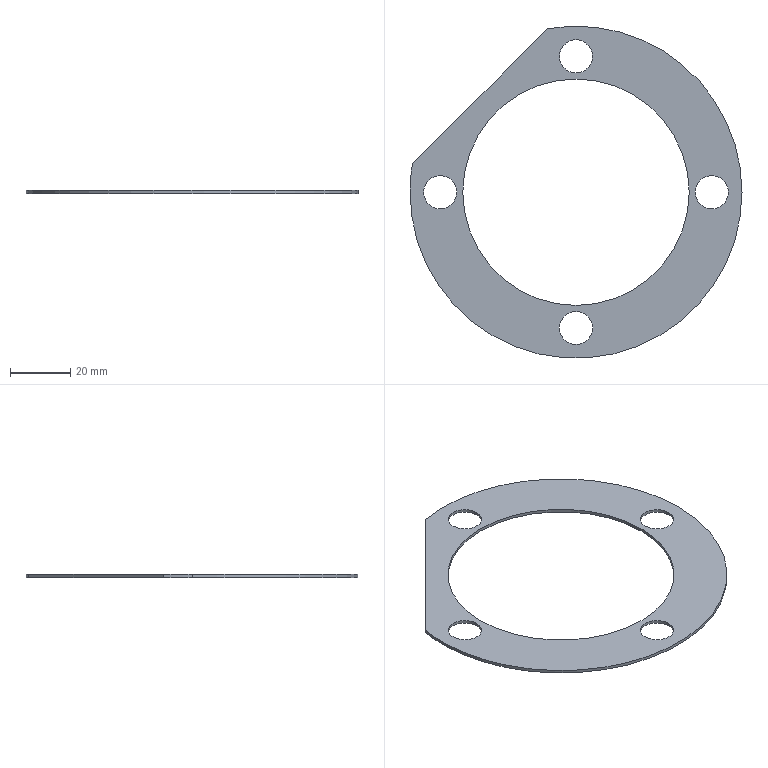Part | SolidWorks | features BaseBody 1 | 1 solid | 16 faces | box 110 x 110 x 1 mm | volume 4275 mm3 | cylinder 13 | plane 3 | commonest cylinder face diameters 11 x8 110 x3 75 x2
STEP:
#1=CARTESIAN_POINT('',(15.5,0.,0.));
#2=VERTEX_POINT('',#1);
#3=CARTESIAN_POINT('',(4.5,0.,0.));
#4=VERTEX_POINT('',#3);
#5=CARTESIAN_POINT('',(10.,0.,0.));
#6=DIRECTION('',(0.,0.,-1.));
#7=DIRECTION('',(1.,0.,0.));
#8=AXIS2_PLACEMENT_3D('',#5,#6,#7);
#9=CIRCLE('',#8,5.5);
#10=EDGE_CURVE('',#2,#4,#9,.T.);
#11=ORIENTED_EDGE('',*,*,#10,.T.);
#12=CARTESIAN_POINT('',(4.5,0.,1.));
#13=VERTEX_POINT('',#12);
#14=CARTESIAN_POINT('',(4.5,0.,0.));
#15=DIRECTION('',(0.,0.,1.));
#16=VECTOR('',#15,1000.);
#17=LINE('',#14,#16);
#18=EDGE_CURVE('',#4,#13,#17,.T.);
#19=ORIENTED_EDGE('',*,*,#18,.T.);
#20=CARTESIAN_POINT('',(15.5,0.,1.));
#21=VERTEX_POINT('',#20);
#22=CARTESIAN_POINT('',(10.,0.,1.));
#23=DIRECTION('',(0.,0.,-1.));
#24=DIRECTION('',(1.,0.,0.));
#25=AXIS2_PLACEMENT_3D('',#22,#23,#24);
#26=CIRCLE('',#25,5.5);
#27=EDGE_CURVE('',#21,#13,#26,.T.);
#28=ORIENTED_EDGE('',*,*,#27,.F.);
#29=CARTESIAN_POINT('',(15.5,0.,0.));
#30=DIRECTION('',(0.,0.,1.));
#31=VECTOR('',#30,1000.);
#32=LINE('',#29,#31);
#33=EDGE_CURVE('',#2,#21,#32,.T.);
#34=ORIENTED_EDGE('',*,*,#33,.F.);
#35=EDGE_LOOP('',(#11,#19,#28,#34));
#36=FACE_OUTER_BOUND('',#35,.T.);
#37=CARTESIAN_POINT('',(10.,0.,0.));
#38=DIRECTION('',(0.,0.,1.));
#39=DIRECTION('',(1.,0.,0.));
#40=AXIS2_PLACEMENT_3D('',#37,#38,#39);
#41=CYLINDRICAL_SURFACE('',#40,5.5);
#42=ADVANCED_FACE('',(#36),#41,.F.);
#43=CARTESIAN_POINT('',(60.5,45.,0.));
#44=VERTEX_POINT('',#43);
#45=CARTESIAN_POINT('',(49.5,45.,0.));
#46=VERTEX_POINT('',#45);
#47=CARTESIAN_POINT('',(55.,45.,0.));
#48=DIRECTION('',(0.,0.,-1.));
#49=DIRECTION('',(1.,0.,0.));
#50=AXIS2_PLACEMENT_3D('',#47,#48,#49);
#51=CIRCLE('',#50,5.5);
#52=EDGE_CURVE('',#44,#46,#51,.T.);
#53=ORIENTED_EDGE('',*,*,#52,.T.);
#54=CARTESIAN_POINT('',(49.5,45.,1.));
#55=VERTEX_POINT('',#54);
#56=CARTESIAN_POINT('',(49.5,45.,0.));
#57=DIRECTION('',(0.,0.,1.));
#58=VECTOR('',#57,1000.);
#59=LINE('',#56,#58);
#60=EDGE_CURVE('',#46,#55,#59,.T.);
#61=ORIENTED_EDGE('',*,*,#60,.T.);
#62=CARTESIAN_POINT('',(60.5,45.,1.));
#63=VERTEX_POINT('',#62);
#64=CARTESIAN_POINT('',(55.,45.,1.));
#65=DIRECTION('',(0.,0.,-1.));
#66=DIRECTION('',(1.,0.,0.));
#67=AXIS2_PLACEMENT_3D('',#64,#65,#66);
#68=CIRCLE('',#67,5.5);
#69=EDGE_CURVE('',#63,#55,#68,.T.);
#70=ORIENTED_EDGE('',*,*,#69,.F.);
#71=CARTESIAN_POINT('',(60.5,45.,0.));
#72=DIRECTION('',(0.,0.,1.));
#73=VECTOR('',#72,1000.);
#74=LINE('',#71,#73);
#75=EDGE_CURVE('',#44,#63,#74,.T.);
#76=ORIENTED_EDGE('',*,*,#75,.F.);
#77=EDGE_LOOP('',(#53,#61,#70,#76));
#78=FACE_OUTER_BOUND('',#77,.T.);
#79=CARTESIAN_POINT('',(55.,45.,0.));
#80=DIRECTION('',(0.,0.,1.));
#81=DIRECTION('',(1.,0.,0.));
#82=AXIS2_PLACEMENT_3D('',#79,#80,#81);
#83=CYLINDRICAL_SURFACE('',#82,5.5);
#84=ADVANCED_FACE('',(#78),#83,.F.);
#85=CARTESIAN_POINT('',(105.5,0.,0.));
#86=VERTEX_POINT('',#85);
#87=CARTESIAN_POINT('',(94.5,0.,0.));
#88=VERTEX_POINT('',#87);
#89=CARTESIAN_POINT('',(100.,0.,0.));
#90=DIRECTION('',(0.,0.,-1.));
#91=DIRECTION('',(1.,0.,0.));
#92=AXIS2_PLACEMENT_3D('',#89,#90,#91);
#93=CIRCLE('',#92,5.5);
#94=EDGE_CURVE('',#86,#88,#93,.T.);
#95=ORIENTED_EDGE('',*,*,#94,.T.);
#96=CARTESIAN_POINT('',(94.5,0.,1.));
#97=VERTEX_POINT('',#96);
#98=CARTESIAN_POINT('',(94.5,0.,0.));
#99=DIRECTION('',(0.,0.,1.));
#100=VECTOR('',#99,1000.);
#101=LINE('',#98,#100);
#102=EDGE_CURVE('',#88,#97,#101,.T.);
#103=ORIENTED_EDGE('',*,*,#102,.T.);
#104=CARTESIAN_POINT('',(105.5,0.,1.));
#105=VERTEX_POINT('',#104);
#106=CARTESIAN_POINT('',(100.,0.,1.));
#107=DIRECTION('',(0.,0.,-1.));
#108=DIRECTION('',(1.,0.,0.));
#109=AXIS2_PLACEMENT_3D('',#106,#107,#108);
#110=CIRCLE('',#109,5.5);
#111=EDGE_CURVE('',#105,#97,#110,.T.);
#112=ORIENTED_EDGE('',*,*,#111,.F.);
#113=CARTESIAN_POINT('',(105.5,0.,0.));
#114=DIRECTION('',(0.,0.,1.));
#115=VECTOR('',#114,1000.);
#116=LINE('',#113,#115);
#117=EDGE_CURVE('',#86,#105,#116,.T.);
#118=ORIENTED_EDGE('',*,*,#117,.F.);
#119=EDGE_LOOP('',(#95,#103,#112,#118));
#120=FACE_OUTER_BOUND('',#119,.T.);
#121=CARTESIAN_POINT('',(100.,0.,0.));
#122=DIRECTION('',(0.,0.,1.));
#123=DIRECTION('',(1.,0.,0.));
#124=AXIS2_PLACEMENT_3D('',#121,#122,#123);
#125=CYLINDRICAL_SURFACE('',#124,5.5);
#126=ADVANCED_FACE('',(#120),#125,.F.);
#127=CARTESIAN_POINT('',(60.5,-45.,0.));
#128=VERTEX_POINT('',#127);
#129=CARTESIAN_POINT('',(49.5,-45.,0.));
#130=VERTEX_POINT('',#129);
#131=CARTESIAN_POINT('',(55.,-45.,0.));
#132=DIRECTION('',(0.,0.,-1.));
#133=DIRECTION('',(1.,0.,0.));
#134=AXIS2_PLACEMENT_3D('',#131,#132,#133);
#135=CIRCLE('',#134,5.5);
#136=EDGE_CURVE('',#128,#130,#135,.T.);
#137=ORIENTED_EDGE('',*,*,#136,.T.);
#138=CARTESIAN_POINT('',(49.5,-45.,1.));
#139=VERTEX_POINT('',#138);
#140=CARTESIAN_POINT('',(49.5,-45.,0.));
#141=DIRECTION('',(0.,0.,1.));
#142=VECTOR('',#141,1000.);
#143=LINE('',#140,#142);
#144=EDGE_CURVE('',#130,#139,#143,.T.);
#145=ORIENTED_EDGE('',*,*,#144,.T.);
#146=CARTESIAN_POINT('',(60.5,-45.,1.));
#147=VERTEX_POINT('',#146);
#148=CARTESIAN_POINT('',(55.,-45.,1.));
#149=DIRECTION('',(0.,0.,-1.));
#150=DIRECTION('',(1.,0.,0.));
#151=AXIS2_PLACEMENT_3D('',#148,#149,#150);
#152=CIRCLE('',#151,5.5);
#153=EDGE_CURVE('',#147,#139,#152,.T.);
#154=ORIENTED_EDGE('',*,*,#153,.F.);
#155=CARTESIAN_POINT('',(60.5,-45.,0.));
#156=DIRECTION('',(0.,0.,1.));
#157=VECTOR('',#156,1000.);
#158=LINE('',#155,#157);
#159=EDGE_CURVE('',#128,#147,#158,.T.);
#160=ORIENTED_EDGE('',*,*,#159,.F.);
#161=EDGE_LOOP('',(#137,#145,#154,#160));
#162=FACE_OUTER_BOUND('',#161,.T.);
#163=CARTESIAN_POINT('',(55.,-45.,0.));
#164=DIRECTION('',(0.,0.,1.));
#165=DIRECTION('',(1.,0.,0.));
#166=AXIS2_PLACEMENT_3D('',#163,#164,#165);
#167=CYLINDRICAL_SURFACE('',#166,5.5);
#168=ADVANCED_FACE('',(#162),#167,.F.);
#169=CARTESIAN_POINT('',(92.5,0.,0.));
#170=VERTEX_POINT('',#169);
#171=CARTESIAN_POINT('',(17.5,0.,0.));
#172=VERTEX_POINT('',#171);
#173=CARTESIAN_POINT('',(55.,0.,0.));
#174=DIRECTION('',(0.,0.,-1.));
#175=DIRECTION('',(1.,0.,0.));
#176=AXIS2_PLACEMENT_3D('',#173,#174,#175);
#177=CIRCLE('',#176,37.5);
#178=EDGE_CURVE('',#170,#172,#177,.T.);
#179=ORIENTED_EDGE('',*,*,#178,.T.);
#180=CARTESIAN_POINT('',(17.5,0.,1.));
#181=VERTEX_POINT('',#180);
#182=CARTESIAN_POINT('',(17.5,0.,0.));
#183=DIRECTION('',(0.,0.,1.));
#184=VECTOR('',#183,1000.);
#185=LINE('',#182,#184);
#186=EDGE_CURVE('',#172,#181,#185,.T.);
#187=ORIENTED_EDGE('',*,*,#186,.T.);
#188=CARTESIAN_POINT('',(92.5,0.,1.));
#189=VERTEX_POINT('',#188);
#190=CARTESIAN_POINT('',(55.,0.,1.));
#191=DIRECTION('',(0.,0.,-1.));
#192=DIRECTION('',(1.,0.,0.));
#193=AXIS2_PLACEMENT_3D('',#190,#191,#192);
#194=CIRCLE('',#193,37.5);
#195=EDGE_CURVE('',#189,#181,#194,.T.);
#196=ORIENTED_EDGE('',*,*,#195,.F.);
#197=CARTESIAN_POINT('',(92.5,0.,0.));
#198=DIRECTION('',(0.,0.,1.));
#199=VECTOR('',#198,1000.);
#200=LINE('',#197,#199);
#201=EDGE_CURVE('',#170,#189,#200,.T.);
#202=ORIENTED_EDGE('',*,*,#201,.F.);
#203=EDGE_LOOP('',(#179,#187,#196,#202));
#204=FACE_OUTER_BOUND('',#203,.T.);
#205=CARTESIAN_POINT('',(55.,0.,0.));
#206=DIRECTION('',(0.,0.,1.));
#207=DIRECTION('',(1.,0.,0.));
#208=AXIS2_PLACEMENT_3D('',#205,#206,#207);
#209=CYLINDRICAL_SURFACE('',#208,37.5);
#210=ADVANCED_FACE('',(#204),#209,.F.);
#211=CARTESIAN_POINT('',(0.8195,9.459,0.));
#212=VERTEX_POINT('',#211);
#213=CARTESIAN_POINT('',(0.,0.,0.));
#214=VERTEX_POINT('',#213);
#215=CARTESIAN_POINT('',(55.,0.,0.));
#216=DIRECTION('',(0.,0.,1.));
#217=DIRECTION('',(1.,0.,0.));
#218=AXIS2_PLACEMENT_3D('',#215,#216,#217);
#219=CIRCLE('',#218,55.);
#220=EDGE_CURVE('',#212,#214,#219,.T.);
#221=ORIENTED_EDGE('',*,*,#220,.T.);
#222=CARTESIAN_POINT('',(0.,0.,1.));
#223=VERTEX_POINT('',#222);
#224=CARTESIAN_POINT('',(0.,0.,0.));
#225=DIRECTION('',(0.,0.,1.));
#226=VECTOR('',#225,1000.);
#227=LINE('',#224,#226);
#228=EDGE_CURVE('',#214,#223,#227,.T.);
#229=ORIENTED_EDGE('',*,*,#228,.T.);
#230=CARTESIAN_POINT('',(0.8195,9.459,1.));
#231=VERTEX_POINT('',#230);
#232=CARTESIAN_POINT('',(55.,0.,1.));
#233=DIRECTION('',(0.,0.,-1.));
#234=DIRECTION('',(1.,0.,0.));
#235=AXIS2_PLACEMENT_3D('',#232,#233,#234);
#236=CIRCLE('',#235,55.);
#237=EDGE_CURVE('',#223,#231,#236,.T.);
#238=ORIENTED_EDGE('',*,*,#237,.T.);
#239=CARTESIAN_POINT('',(0.8195,9.459,0.));
#240=DIRECTION('',(0.,0.,1.));
#241=VECTOR('',#240,1000.);
#242=LINE('',#239,#241);
#243=EDGE_CURVE('',#212,#231,#242,.T.);
#244=ORIENTED_EDGE('',*,*,#243,.F.);
#245=EDGE_LOOP('',(#221,#229,#238,#244));
#246=FACE_OUTER_BOUND('',#245,.T.);
#247=CARTESIAN_POINT('',(55.,0.,0.));
#248=DIRECTION('',(0.,0.,1.));
#249=DIRECTION('',(1.,0.,0.));
#250=AXIS2_PLACEMENT_3D('',#247,#248,#249);
#251=CYLINDRICAL_SURFACE('',#250,55.);
#252=ADVANCED_FACE('',(#246),#251,.T.);
#253=ORIENTED_EDGE('',*,*,#228,.F.);
#254=CARTESIAN_POINT('',(110.,0.,0.));
#255=VERTEX_POINT('',#254);
#256=CARTESIAN_POINT('',(55.,0.,0.));
#257=DIRECTION('',(0.,0.,1.));
#258=DIRECTION('',(1.,0.,0.));
#259=AXIS2_PLACEMENT_3D('',#256,#257,#258);
#260=CIRCLE('',#259,55.);
#261=EDGE_CURVE('',#214,#255,#260,.T.);
#262=ORIENTED_EDGE('',*,*,#261,.T.);
#263=CARTESIAN_POINT('',(110.,0.,1.));
#264=VERTEX_POINT('',#263);
#265=CARTESIAN_POINT('',(110.,0.,0.));
#266=DIRECTION('',(0.,0.,1.));
#267=VECTOR('',#266,1000.);
#268=LINE('',#265,#267);
#269=EDGE_CURVE('',#255,#264,#268,.T.);
#270=ORIENTED_EDGE('',*,*,#269,.T.);
#271=CARTESIAN_POINT('',(55.,0.,1.));
#272=DIRECTION('',(0.,0.,-1.));
#273=DIRECTION('',(1.,0.,0.));
#274=AXIS2_PLACEMENT_3D('',#271,#272,#273);
#275=CIRCLE('',#274,55.);
#276=EDGE_CURVE('',#264,#223,#275,.T.);
#277=ORIENTED_EDGE('',*,*,#276,.T.);
#278=EDGE_LOOP('',(#253,#262,#270,#277));
#279=FACE_OUTER_BOUND('',#278,.T.);
#280=CARTESIAN_POINT('',(55.,0.,0.));
#281=DIRECTION('',(0.,0.,1.));
#282=DIRECTION('',(1.,0.,0.));
#283=AXIS2_PLACEMENT_3D('',#280,#281,#282);
#284=CYLINDRICAL_SURFACE('',#283,55.);
#285=ADVANCED_FACE('',(#279),#284,.T.);
#286=ORIENTED_EDGE('',*,*,#10,.F.);
#287=CARTESIAN_POINT('',(10.,0.,0.));
#288=DIRECTION('',(0.,0.,-1.));
#289=DIRECTION('',(1.,0.,0.));
#290=AXIS2_PLACEMENT_3D('',#287,#288,#289);
#291=CIRCLE('',#290,5.5);
#292=EDGE_CURVE('',#4,#2,#291,.T.);
#293=ORIENTED_EDGE('',*,*,#292,.F.);
#294=EDGE_LOOP('',(#286,#293));
#295=FACE_BOUND('',#294,.T.);
#296=ORIENTED_EDGE('',*,*,#52,.F.);
#297=CARTESIAN_POINT('',(55.,45.,0.));
#298=DIRECTION('',(0.,0.,-1.));
#299=DIRECTION('',(1.,0.,0.));
#300=AXIS2_PLACEMENT_3D('',#297,#298,#299);
#301=CIRCLE('',#300,5.5);
#302=EDGE_CURVE('',#46,#44,#301,.T.);
#303=ORIENTED_EDGE('',*,*,#302,.F.);
#304=EDGE_LOOP('',(#296,#303));
#305=FACE_BOUND('',#304,.T.);
#306=ORIENTED_EDGE('',*,*,#94,.F.);
#307=CARTESIAN_POINT('',(100.,0.,0.));
#308=DIRECTION('',(0.,0.,-1.));
#309=DIRECTION('',(1.,0.,0.));
#310=AXIS2_PLACEMENT_3D('',#307,#308,#309);
#311=CIRCLE('',#310,5.5);
#312=EDGE_CURVE('',#88,#86,#311,.T.);
#313=ORIENTED_EDGE('',*,*,#312,.F.);
#314=EDGE_LOOP('',(#306,#313));
#315=FACE_BOUND('',#314,.T.);
#316=ORIENTED_EDGE('',*,*,#136,.F.);
#317=CARTESIAN_POINT('',(55.,-45.,0.));
#318=DIRECTION('',(0.,0.,-1.));
#319=DIRECTION('',(1.,0.,0.));
#320=AXIS2_PLACEMENT_3D('',#317,#318,#319);
#321=CIRCLE('',#320,5.5);
#322=EDGE_CURVE('',#130,#128,#321,.T.);
#323=ORIENTED_EDGE('',*,*,#322,.F.);
#324=EDGE_LOOP('',(#316,#323));
#325=FACE_BOUND('',#324,.T.);
#326=ORIENTED_EDGE('',*,*,#178,.F.);
#327=CARTESIAN_POINT('',(55.,0.,0.));
#328=DIRECTION('',(0.,0.,-1.));
#329=DIRECTION('',(1.,0.,0.));
#330=AXIS2_PLACEMENT_3D('',#327,#328,#329);
#331=CIRCLE('',#330,37.5);
#332=EDGE_CURVE('',#172,#170,#331,.T.);
#333=ORIENTED_EDGE('',*,*,#332,.F.);
#334=EDGE_LOOP('',(#326,#333));
#335=FACE_BOUND('',#334,.T.);
#336=ORIENTED_EDGE('',*,*,#220,.F.);
#337=CARTESIAN_POINT('',(45.541,54.18,0.));
#338=VERTEX_POINT('',#337);
#339=CARTESIAN_POINT('',(45.541,54.18,0.));
#340=DIRECTION('',(-0.7071,-0.7071,0.));
#341=VECTOR('',#340,1000.);
#342=LINE('',#339,#341);
#343=EDGE_CURVE('',#338,#212,#342,.T.);
#344=ORIENTED_EDGE('',*,*,#343,.F.);
#345=CARTESIAN_POINT('',(55.,0.,0.));
#346=DIRECTION('',(0.,0.,1.));
#347=DIRECTION('',(1.,0.,0.));
#348=AXIS2_PLACEMENT_3D('',#345,#346,#347);
#349=CIRCLE('',#348,55.);
#350=EDGE_CURVE('',#255,#338,#349,.T.);
#351=ORIENTED_EDGE('',*,*,#350,.F.);
#352=ORIENTED_EDGE('',*,*,#261,.F.);
#353=EDGE_LOOP('',(#336,#344,#351,#352));
#354=FACE_OUTER_BOUND('',#353,.T.);
#355=CARTESIAN_POINT('',(54.383,0.6168,0.));
#356=DIRECTION('',(0.,0.,1.));
#357=DIRECTION('',(1.,0.,0.));
#358=AXIS2_PLACEMENT_3D('',#355,#356,#357);
#359=PLANE('',#358);
#360=ADVANCED_FACE('',(#295,#305,#315,#325,#335,#354),#359,.F.);
#361=ORIENTED_EDGE('',*,*,#18,.F.);
#362=ORIENTED_EDGE('',*,*,#292,.T.);
#363=ORIENTED_EDGE('',*,*,#33,.T.);
#364=CARTESIAN_POINT('',(10.,0.,1.));
#365=DIRECTION('',(0.,0.,-1.));
#366=DIRECTION('',(1.,0.,0.));
#367=AXIS2_PLACEMENT_3D('',#364,#365,#366);
#368=CIRCLE('',#367,5.5);
#369=EDGE_CURVE('',#13,#21,#368,.T.);
#370=ORIENTED_EDGE('',*,*,#369,.F.);
#371=EDGE_LOOP('',(#361,#362,#363,#370));
#372=FACE_OUTER_BOUND('',#371,.T.);
#373=CARTESIAN_POINT('',(10.,0.,0.));
#374=DIRECTION('',(0.,0.,1.));
#375=DIRECTION('',(1.,0.,0.));
#376=AXIS2_PLACEMENT_3D('',#373,#374,#375);
#377=CYLINDRICAL_SURFACE('',#376,5.5);
#378=ADVANCED_FACE('',(#372),#377,.F.);
#379=ORIENTED_EDGE('',*,*,#60,.F.);
#380=ORIENTED_EDGE('',*,*,#302,.T.);
#381=ORIENTED_EDGE('',*,*,#75,.T.);
#382=CARTESIAN_POINT('',(55.,45.,1.));
#383=DIRECTION('',(0.,0.,-1.));
#384=DIRECTION('',(1.,0.,0.));
#385=AXIS2_PLACEMENT_3D('',#382,#383,#384);
#386=CIRCLE('',#385,5.5);
#387=EDGE_CURVE('',#55,#63,#386,.T.);
#388=ORIENTED_EDGE('',*,*,#387,.F.);
#389=EDGE_LOOP('',(#379,#380,#381,#388));
#390=FACE_OUTER_BOUND('',#389,.T.);
#391=CARTESIAN_POINT('',(55.,45.,0.));
#392=DIRECTION('',(0.,0.,1.));
#393=DIRECTION('',(1.,0.,0.));
#394=AXIS2_PLACEMENT_3D('',#391,#392,#393);
#395=CYLINDRICAL_SURFACE('',#394,5.5);
#396=ADVANCED_FACE('',(#390),#395,.F.);
#397=ORIENTED_EDGE('',*,*,#102,.F.);
#398=ORIENTED_EDGE('',*,*,#312,.T.);
#399=ORIENTED_EDGE('',*,*,#117,.T.);
#400=CARTESIAN_POINT('',(100.,0.,1.));
#401=DIRECTION('',(0.,0.,-1.));
#402=DIRECTION('',(1.,0.,0.));
#403=AXIS2_PLACEMENT_3D('',#400,#401,#402);
#404=CIRCLE('',#403,5.5);
#405=EDGE_CURVE('',#97,#105,#404,.T.);
#406=ORIENTED_EDGE('',*,*,#405,.F.);
#407=EDGE_LOOP('',(#397,#398,#399,#406));
#408=FACE_OUTER_BOUND('',#407,.T.);
#409=CARTESIAN_POINT('',(100.,0.,0.));
#410=DIRECTION('',(0.,0.,1.));
#411=DIRECTION('',(1.,0.,0.));
#412=AXIS2_PLACEMENT_3D('',#409,#410,#411);
#413=CYLINDRICAL_SURFACE('',#412,5.5);
#414=ADVANCED_FACE('',(#408),#413,.F.);
#415=ORIENTED_EDGE('',*,*,#144,.F.);
#416=ORIENTED_EDGE('',*,*,#322,.T.);
#417=ORIENTED_EDGE('',*,*,#159,.T.);
#418=CARTESIAN_POINT('',(55.,-45.,1.));
#419=DIRECTION('',(0.,0.,-1.));
#420=DIRECTION('',(1.,0.,0.));
#421=AXIS2_PLACEMENT_3D('',#418,#419,#420);
#422=CIRCLE('',#421,5.5);
#423=EDGE_CURVE('',#139,#147,#422,.T.);
#424=ORIENTED_EDGE('',*,*,#423,.F.);
#425=EDGE_LOOP('',(#415,#416,#417,#424));
#426=FACE_OUTER_BOUND('',#425,.T.);
#427=CARTESIAN_POINT('',(55.,-45.,0.));
#428=DIRECTION('',(0.,0.,1.));
#429=DIRECTION('',(1.,0.,0.));
#430=AXIS2_PLACEMENT_3D('',#427,#428,#429);
#431=CYLINDRICAL_SURFACE('',#430,5.5);
#432=ADVANCED_FACE('',(#426),#431,.F.);
#433=ORIENTED_EDGE('',*,*,#186,.F.);
#434=ORIENTED_EDGE('',*,*,#332,.T.);
#435=ORIENTED_EDGE('',*,*,#201,.T.);
#436=CARTESIAN_POINT('',(55.,0.,1.));
#437=DIRECTION('',(0.,0.,-1.));
#438=DIRECTION('',(1.,0.,0.));
#439=AXIS2_PLACEMENT_3D('',#436,#437,#438);
#440=CIRCLE('',#439,37.5);
#441=EDGE_CURVE('',#181,#189,#440,.T.);
#442=ORIENTED_EDGE('',*,*,#441,.F.);
#443=EDGE_LOOP('',(#433,#434,#435,#442));
#444=FACE_OUTER_BOUND('',#443,.T.);
#445=CARTESIAN_POINT('',(55.,0.,0.));
#446=DIRECTION('',(0.,0.,1.));
#447=DIRECTION('',(1.,0.,0.));
#448=AXIS2_PLACEMENT_3D('',#445,#446,#447);
#449=CYLINDRICAL_SURFACE('',#448,37.5);
#450=ADVANCED_FACE('',(#444),#449,.F.);
#451=CARTESIAN_POINT('',(45.541,54.18,1.));
#452=VERTEX_POINT('',#451);
#453=CARTESIAN_POINT('',(45.541,54.18,1.));
#454=DIRECTION('',(0.7071,0.7071,0.));
#455=VECTOR('',#454,1000.);
#456=LINE('',#453,#455);
#457=EDGE_CURVE('',#231,#452,#456,.T.);
#458=ORIENTED_EDGE('',*,*,#457,.T.);
#459=CARTESIAN_POINT('',(45.541,54.18,0.));
#460=DIRECTION('',(0.,0.,-1.));
#461=VECTOR('',#460,1000.);
#462=LINE('',#459,#461);
#463=EDGE_CURVE('',#452,#338,#462,.T.);
#464=ORIENTED_EDGE('',*,*,#463,.T.);
#465=ORIENTED_EDGE('',*,*,#343,.T.);
#466=ORIENTED_EDGE('',*,*,#243,.T.);
#467=EDGE_LOOP('',(#458,#464,#465,#466));
#468=FACE_OUTER_BOUND('',#467,.T.);
#469=CARTESIAN_POINT('',(45.541,54.18,0.));
#470=DIRECTION('',(-0.7071,0.7071,0.));
#471=DIRECTION('',(-0.7071,-0.7071,0.));
#472=AXIS2_PLACEMENT_3D('',#469,#470,#471);
#473=PLANE('',#472);
#474=ADVANCED_FACE('',(#468),#473,.T.);
#475=ORIENTED_EDGE('',*,*,#269,.F.);
#476=ORIENTED_EDGE('',*,*,#350,.T.);
#477=ORIENTED_EDGE('',*,*,#463,.F.);
#478=CARTESIAN_POINT('',(55.,0.,1.));
#479=DIRECTION('',(0.,0.,-1.));
#480=DIRECTION('',(1.,0.,0.));
#481=AXIS2_PLACEMENT_3D('',#478,#479,#480);
#482=CIRCLE('',#481,55.);
#483=EDGE_CURVE('',#452,#264,#482,.T.);
#484=ORIENTED_EDGE('',*,*,#483,.T.);
#485=EDGE_LOOP('',(#475,#476,#477,#484));
#486=FACE_OUTER_BOUND('',#485,.T.);
#487=CARTESIAN_POINT('',(55.,0.,0.));
#488=DIRECTION('',(0.,0.,1.));
#489=DIRECTION('',(1.,0.,0.));
#490=AXIS2_PLACEMENT_3D('',#487,#488,#489);
#491=CYLINDRICAL_SURFACE('',#490,55.);
#492=ADVANCED_FACE('',(#486),#491,.T.);
#493=ORIENTED_EDGE('',*,*,#27,.T.);
#494=ORIENTED_EDGE('',*,*,#369,.T.);
#495=EDGE_LOOP('',(#493,#494));
#496=FACE_BOUND('',#495,.T.);
#497=ORIENTED_EDGE('',*,*,#69,.T.);
#498=ORIENTED_EDGE('',*,*,#387,.T.);
#499=EDGE_LOOP('',(#497,#498));
#500=FACE_BOUND('',#499,.T.);
#501=ORIENTED_EDGE('',*,*,#111,.T.);
#502=ORIENTED_EDGE('',*,*,#405,.T.);
#503=EDGE_LOOP('',(#501,#502));
#504=FACE_BOUND('',#503,.T.);
#505=ORIENTED_EDGE('',*,*,#153,.T.);
#506=ORIENTED_EDGE('',*,*,#423,.T.);
#507=EDGE_LOOP('',(#505,#506));
#508=FACE_BOUND('',#507,.T.);
#509=ORIENTED_EDGE('',*,*,#195,.T.);
#510=ORIENTED_EDGE('',*,*,#441,.T.);
#511=EDGE_LOOP('',(#509,#510));
#512=FACE_BOUND('',#511,.T.);
#513=ORIENTED_EDGE('',*,*,#457,.F.);
#514=ORIENTED_EDGE('',*,*,#237,.F.);
#515=ORIENTED_EDGE('',*,*,#276,.F.);
#516=ORIENTED_EDGE('',*,*,#483,.F.);
#517=EDGE_LOOP('',(#513,#514,#515,#516));
#518=FACE_OUTER_BOUND('',#517,.T.);
#519=CARTESIAN_POINT('',(54.383,0.6168,1.));
#520=DIRECTION('',(0.,0.,1.));
#521=DIRECTION('',(1.,0.,0.));
#522=AXIS2_PLACEMENT_3D('',#519,#520,#521);
#523=PLANE('',#522);
#524=ADVANCED_FACE('',(#496,#500,#504,#508,#512,#518),#523,.T.);
#525=CLOSED_SHELL('',(#42,#84,#126,#168,#210,#252,#285,#360,#378,#396,#414,#432,#450,#474,#492,#524));
#526=MANIFOLD_SOLID_BREP('',#525);
#527=CARTESIAN_POINT('',(0.,0.,0.));
#528=DIRECTION('',(0.,0.,1.));
#529=DIRECTION('',(1.,0.,0.));
#530=AXIS2_PLACEMENT_3D('',#527,#528,#529);
#531=(LENGTH_UNIT()NAMED_UNIT(*)SI_UNIT(.MILLI.,.METRE.));
#532=UNCERTAINTY_MEASURE_WITH_UNIT(LENGTH_MEASURE(0.00001),#531,'','');
#533=(NAMED_UNIT(*)PLANE_ANGLE_UNIT()SI_UNIT($,.RADIAN.));
#534=(NAMED_UNIT(*)SI_UNIT($,.STERADIAN.)SOLID_ANGLE_UNIT());
#535=(GEOMETRIC_REPRESENTATION_CONTEXT(3)GLOBAL_UNCERTAINTY_ASSIGNED_CONTEXT((#532))GLOBAL_UNIT_ASSIGNED_CONTEXT((#531,#533,#534))REPRESENTATION_CONTEXT('',''));
#536=ADVANCED_BREP_SHAPE_REPRESENTATION('',(#526,#530),#535);